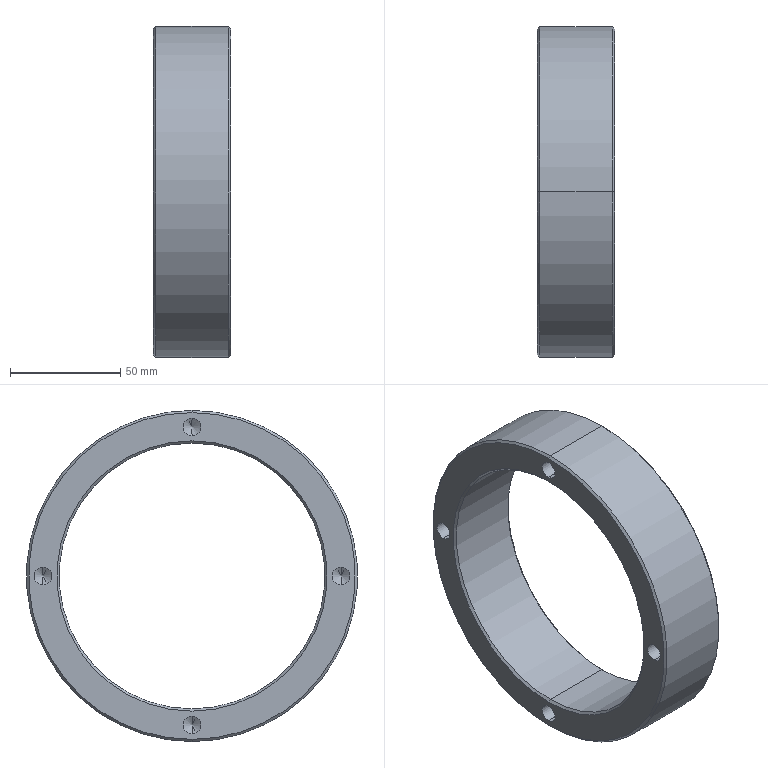Part | SolidWorks | features Chamfer 1, Extrusion 1, HoleWzd 1 | 1 solid | 30 faces | box 35 x 150 x 150 mm | volume 215991 mm3 | cone 16 | cylinder 12 | plane 2 | commonest cylinder face diameters 8 x8 120.4 x2 150 x2
STEP:
#1=CARTESIAN_POINT('',(15.,67.5,-4.));
#2=VERTEX_POINT('',#1);
#3=CARTESIAN_POINT('',(15.,67.5,4.));
#4=VERTEX_POINT('',#3);
#5=CARTESIAN_POINT('',(15.,67.5,0.));
#6=DIRECTION('',(-1.,0.,0.));
#7=DIRECTION('',(0.,0.,1.));
#8=AXIS2_PLACEMENT_3D('',#5,#6,#7);
#9=CIRCLE('',#8,4.);
#10=EDGE_CURVE('',#2,#4,#9,.T.);
#11=ORIENTED_EDGE('',*,*,#10,.F.);
#12=CARTESIAN_POINT('',(0.,67.5,-4.));
#13=VERTEX_POINT('',#12);
#14=CARTESIAN_POINT('',(0.,67.5,-4.));
#15=DIRECTION('',(-1.,0.,0.));
#16=VECTOR('',#15,1000.);
#17=LINE('',#14,#16);
#18=EDGE_CURVE('',#2,#13,#17,.T.);
#19=ORIENTED_EDGE('',*,*,#18,.T.);
#20=CARTESIAN_POINT('',(0.,67.5,4.));
#21=VERTEX_POINT('',#20);
#22=CARTESIAN_POINT('',(0.,67.5,0.));
#23=DIRECTION('',(-1.,0.,0.));
#24=DIRECTION('',(0.,0.,1.));
#25=AXIS2_PLACEMENT_3D('',#22,#23,#24);
#26=CIRCLE('',#25,4.);
#27=EDGE_CURVE('',#13,#21,#26,.T.);
#28=ORIENTED_EDGE('',*,*,#27,.T.);
#29=CARTESIAN_POINT('',(0.,67.5,4.));
#30=DIRECTION('',(-1.,0.,0.));
#31=VECTOR('',#30,1000.);
#32=LINE('',#29,#31);
#33=EDGE_CURVE('',#4,#21,#32,.T.);
#34=ORIENTED_EDGE('',*,*,#33,.F.);
#35=EDGE_LOOP('',(#11,#19,#28,#34));
#36=FACE_OUTER_BOUND('',#35,.T.);
#37=CARTESIAN_POINT('',(0.,67.5,0.));
#38=DIRECTION('',(-1.,0.,0.));
#39=DIRECTION('',(0.,0.,1.));
#40=AXIS2_PLACEMENT_3D('',#37,#38,#39);
#41=CYLINDRICAL_SURFACE('',#40,4.);
#42=ADVANCED_FACE('',(#36),#41,.F.);
#43=CARTESIAN_POINT('',(17.403,67.5,0.));
#44=VERTEX_POINT('',#43);
#45=CARTESIAN_POINT('',(15.,67.5,4.));
#46=DIRECTION('',(-0.515,0.,0.8572));
#47=VECTOR('',#46,1000.);
#48=LINE('',#45,#47);
#49=EDGE_CURVE('',#44,#4,#48,.T.);
#50=ORIENTED_EDGE('',*,*,#49,.F.);
#51=CARTESIAN_POINT('',(15.,67.5,-4.));
#52=DIRECTION('',(-0.515,0.,-0.8572));
#53=VECTOR('',#52,1000.);
#54=LINE('',#51,#53);
#55=EDGE_CURVE('',#44,#2,#54,.T.);
#56=ORIENTED_EDGE('',*,*,#55,.T.);
#57=ORIENTED_EDGE('',*,*,#10,.T.);
#58=EDGE_LOOP('',(#50,#56,#57));
#59=FACE_OUTER_BOUND('',#58,.T.);
#60=CARTESIAN_POINT('',(15.,67.5,0.));
#61=DIRECTION('',(-1.,0.,0.));
#62=DIRECTION('',(0.,0.,1.));
#63=AXIS2_PLACEMENT_3D('',#60,#61,#62);
#64=CONICAL_SURFACE('',#63,4.,1.03);
#65=ADVANCED_FACE('',(#59),#64,.F.);
#66=CARTESIAN_POINT('',(15.,0.,63.5));
#67=VERTEX_POINT('',#66);
#68=CARTESIAN_POINT('',(15.,0.,71.5));
#69=VERTEX_POINT('',#68);
#70=CARTESIAN_POINT('',(15.,0.,67.5));
#71=DIRECTION('',(-1.,0.,0.));
#72=DIRECTION('',(0.,0.,1.));
#73=AXIS2_PLACEMENT_3D('',#70,#71,#72);
#74=CIRCLE('',#73,4.);
#75=EDGE_CURVE('',#67,#69,#74,.T.);
#76=ORIENTED_EDGE('',*,*,#75,.F.);
#77=CARTESIAN_POINT('',(0.,0.,63.5));
#78=VERTEX_POINT('',#77);
#79=CARTESIAN_POINT('',(0.,0.,63.5));
#80=DIRECTION('',(-1.,0.,0.));
#81=VECTOR('',#80,1000.);
#82=LINE('',#79,#81);
#83=EDGE_CURVE('',#67,#78,#82,.T.);
#84=ORIENTED_EDGE('',*,*,#83,.T.);
#85=CARTESIAN_POINT('',(0.,0.,71.5));
#86=VERTEX_POINT('',#85);
#87=CARTESIAN_POINT('',(0.,0.,67.5));
#88=DIRECTION('',(-1.,0.,0.));
#89=DIRECTION('',(0.,0.,1.));
#90=AXIS2_PLACEMENT_3D('',#87,#88,#89);
#91=CIRCLE('',#90,4.);
#92=EDGE_CURVE('',#78,#86,#91,.T.);
#93=ORIENTED_EDGE('',*,*,#92,.T.);
#94=CARTESIAN_POINT('',(0.,0.,71.5));
#95=DIRECTION('',(-1.,0.,0.));
#96=VECTOR('',#95,1000.);
#97=LINE('',#94,#96);
#98=EDGE_CURVE('',#69,#86,#97,.T.);
#99=ORIENTED_EDGE('',*,*,#98,.F.);
#100=EDGE_LOOP('',(#76,#84,#93,#99));
#101=FACE_OUTER_BOUND('',#100,.T.);
#102=CARTESIAN_POINT('',(0.,0.,67.5));
#103=DIRECTION('',(-1.,0.,0.));
#104=DIRECTION('',(0.,0.,1.));
#105=AXIS2_PLACEMENT_3D('',#102,#103,#104);
#106=CYLINDRICAL_SURFACE('',#105,4.);
#107=ADVANCED_FACE('',(#101),#106,.F.);
#108=CARTESIAN_POINT('',(17.403,0.,67.5));
#109=VERTEX_POINT('',#108);
#110=CARTESIAN_POINT('',(15.,0.,71.5));
#111=DIRECTION('',(-0.515,0.,0.8572));
#112=VECTOR('',#111,1000.);
#113=LINE('',#110,#112);
#114=EDGE_CURVE('',#109,#69,#113,.T.);
#115=ORIENTED_EDGE('',*,*,#114,.F.);
#116=CARTESIAN_POINT('',(15.,0.,63.5));
#117=DIRECTION('',(-0.515,0.,-0.8572));
#118=VECTOR('',#117,1000.);
#119=LINE('',#116,#118);
#120=EDGE_CURVE('',#109,#67,#119,.T.);
#121=ORIENTED_EDGE('',*,*,#120,.T.);
#122=ORIENTED_EDGE('',*,*,#75,.T.);
#123=EDGE_LOOP('',(#115,#121,#122));
#124=FACE_OUTER_BOUND('',#123,.T.);
#125=CARTESIAN_POINT('',(15.,0.,67.5));
#126=DIRECTION('',(-1.,0.,0.));
#127=DIRECTION('',(0.,0.,1.));
#128=AXIS2_PLACEMENT_3D('',#125,#126,#127);
#129=CONICAL_SURFACE('',#128,4.,1.03);
#130=ADVANCED_FACE('',(#124),#129,.F.);
#131=CARTESIAN_POINT('',(15.,-67.5,-4.));
#132=VERTEX_POINT('',#131);
#133=CARTESIAN_POINT('',(15.,-67.5,4.));
#134=VERTEX_POINT('',#133);
#135=CARTESIAN_POINT('',(15.,-67.5,0.));
#136=DIRECTION('',(-1.,0.,0.));
#137=DIRECTION('',(0.,0.,1.));
#138=AXIS2_PLACEMENT_3D('',#135,#136,#137);
#139=CIRCLE('',#138,4.);
#140=EDGE_CURVE('',#132,#134,#139,.T.);
#141=ORIENTED_EDGE('',*,*,#140,.F.);
#142=CARTESIAN_POINT('',(0.,-67.5,-4.));
#143=VERTEX_POINT('',#142);
#144=CARTESIAN_POINT('',(0.,-67.5,-4.));
#145=DIRECTION('',(-1.,0.,0.));
#146=VECTOR('',#145,1000.);
#147=LINE('',#144,#146);
#148=EDGE_CURVE('',#132,#143,#147,.T.);
#149=ORIENTED_EDGE('',*,*,#148,.T.);
#150=CARTESIAN_POINT('',(0.,-67.5,4.));
#151=VERTEX_POINT('',#150);
#152=CARTESIAN_POINT('',(0.,-67.5,0.));
#153=DIRECTION('',(-1.,0.,0.));
#154=DIRECTION('',(0.,0.,1.));
#155=AXIS2_PLACEMENT_3D('',#152,#153,#154);
#156=CIRCLE('',#155,4.);
#157=EDGE_CURVE('',#143,#151,#156,.T.);
#158=ORIENTED_EDGE('',*,*,#157,.T.);
#159=CARTESIAN_POINT('',(0.,-67.5,4.));
#160=DIRECTION('',(-1.,0.,0.));
#161=VECTOR('',#160,1000.);
#162=LINE('',#159,#161);
#163=EDGE_CURVE('',#134,#151,#162,.T.);
#164=ORIENTED_EDGE('',*,*,#163,.F.);
#165=EDGE_LOOP('',(#141,#149,#158,#164));
#166=FACE_OUTER_BOUND('',#165,.T.);
#167=CARTESIAN_POINT('',(0.,-67.5,0.));
#168=DIRECTION('',(-1.,0.,0.));
#169=DIRECTION('',(0.,0.,1.));
#170=AXIS2_PLACEMENT_3D('',#167,#168,#169);
#171=CYLINDRICAL_SURFACE('',#170,4.);
#172=ADVANCED_FACE('',(#166),#171,.F.);
#173=CARTESIAN_POINT('',(17.403,-67.5,0.));
#174=VERTEX_POINT('',#173);
#175=CARTESIAN_POINT('',(15.,-67.5,4.));
#176=DIRECTION('',(-0.515,0.,0.8572));
#177=VECTOR('',#176,1000.);
#178=LINE('',#175,#177);
#179=EDGE_CURVE('',#174,#134,#178,.T.);
#180=ORIENTED_EDGE('',*,*,#179,.F.);
#181=CARTESIAN_POINT('',(15.,-67.5,-4.));
#182=DIRECTION('',(-0.515,0.,-0.8572));
#183=VECTOR('',#182,1000.);
#184=LINE('',#181,#183);
#185=EDGE_CURVE('',#174,#132,#184,.T.);
#186=ORIENTED_EDGE('',*,*,#185,.T.);
#187=ORIENTED_EDGE('',*,*,#140,.T.);
#188=EDGE_LOOP('',(#180,#186,#187));
#189=FACE_OUTER_BOUND('',#188,.T.);
#190=CARTESIAN_POINT('',(15.,-67.5,0.));
#191=DIRECTION('',(-1.,0.,0.));
#192=DIRECTION('',(0.,0.,1.));
#193=AXIS2_PLACEMENT_3D('',#190,#191,#192);
#194=CONICAL_SURFACE('',#193,4.,1.03);
#195=ADVANCED_FACE('',(#189),#194,.F.);
#196=CARTESIAN_POINT('',(15.,0.,-71.5));
#197=VERTEX_POINT('',#196);
#198=CARTESIAN_POINT('',(15.,0.,-63.5));
#199=VERTEX_POINT('',#198);
#200=CARTESIAN_POINT('',(15.,0.,-67.5));
#201=DIRECTION('',(-1.,0.,0.));
#202=DIRECTION('',(0.,0.,1.));
#203=AXIS2_PLACEMENT_3D('',#200,#201,#202);
#204=CIRCLE('',#203,4.);
#205=EDGE_CURVE('',#197,#199,#204,.T.);
#206=ORIENTED_EDGE('',*,*,#205,.F.);
#207=CARTESIAN_POINT('',(0.,0.,-71.5));
#208=VERTEX_POINT('',#207);
#209=CARTESIAN_POINT('',(0.,0.,-71.5));
#210=DIRECTION('',(-1.,0.,0.));
#211=VECTOR('',#210,1000.);
#212=LINE('',#209,#211);
#213=EDGE_CURVE('',#197,#208,#212,.T.);
#214=ORIENTED_EDGE('',*,*,#213,.T.);
#215=CARTESIAN_POINT('',(0.,0.,-63.5));
#216=VERTEX_POINT('',#215);
#217=CARTESIAN_POINT('',(0.,0.,-67.5));
#218=DIRECTION('',(-1.,0.,0.));
#219=DIRECTION('',(0.,0.,1.));
#220=AXIS2_PLACEMENT_3D('',#217,#218,#219);
#221=CIRCLE('',#220,4.);
#222=EDGE_CURVE('',#208,#216,#221,.T.);
#223=ORIENTED_EDGE('',*,*,#222,.T.);
#224=CARTESIAN_POINT('',(0.,0.,-63.5));
#225=DIRECTION('',(-1.,0.,0.));
#226=VECTOR('',#225,1000.);
#227=LINE('',#224,#226);
#228=EDGE_CURVE('',#199,#216,#227,.T.);
#229=ORIENTED_EDGE('',*,*,#228,.F.);
#230=EDGE_LOOP('',(#206,#214,#223,#229));
#231=FACE_OUTER_BOUND('',#230,.T.);
#232=CARTESIAN_POINT('',(0.,0.,-67.5));
#233=DIRECTION('',(-1.,0.,0.));
#234=DIRECTION('',(0.,0.,1.));
#235=AXIS2_PLACEMENT_3D('',#232,#233,#234);
#236=CYLINDRICAL_SURFACE('',#235,4.);
#237=ADVANCED_FACE('',(#231),#236,.F.);
#238=CARTESIAN_POINT('',(17.403,0.,-67.5));
#239=VERTEX_POINT('',#238);
#240=CARTESIAN_POINT('',(15.,0.,-63.5));
#241=DIRECTION('',(-0.515,0.,0.8572));
#242=VECTOR('',#241,1000.);
#243=LINE('',#240,#242);
#244=EDGE_CURVE('',#239,#199,#243,.T.);
#245=ORIENTED_EDGE('',*,*,#244,.F.);
#246=CARTESIAN_POINT('',(15.,0.,-71.5));
#247=DIRECTION('',(-0.515,0.,-0.8572));
#248=VECTOR('',#247,1000.);
#249=LINE('',#246,#248);
#250=EDGE_CURVE('',#239,#197,#249,.T.);
#251=ORIENTED_EDGE('',*,*,#250,.T.);
#252=ORIENTED_EDGE('',*,*,#205,.T.);
#253=EDGE_LOOP('',(#245,#251,#252));
#254=FACE_OUTER_BOUND('',#253,.T.);
#255=CARTESIAN_POINT('',(15.,0.,-67.5));
#256=DIRECTION('',(-1.,0.,0.));
#257=DIRECTION('',(0.,0.,1.));
#258=AXIS2_PLACEMENT_3D('',#255,#256,#257);
#259=CONICAL_SURFACE('',#258,4.,1.03);
#260=ADVANCED_FACE('',(#254),#259,.F.);
#261=CARTESIAN_POINT('',(35.,0.,-74.));
#262=VERTEX_POINT('',#261);
#263=CARTESIAN_POINT('',(35.,0.,74.));
#264=VERTEX_POINT('',#263);
#265=CARTESIAN_POINT('',(35.,0.,0.));
#266=DIRECTION('',(1.,0.,0.));
#267=DIRECTION('',(0.,0.,-1.));
#268=AXIS2_PLACEMENT_3D('',#265,#266,#267);
#269=CIRCLE('',#268,74.);
#270=EDGE_CURVE('',#262,#264,#269,.T.);
#271=ORIENTED_EDGE('',*,*,#270,.F.);
#272=CARTESIAN_POINT('',(34.,0.,-75.));
#273=VERTEX_POINT('',#272);
#274=CARTESIAN_POINT('',(35.,0.,-74.));
#275=DIRECTION('',(-0.7071,0.,-0.7071));
#276=VECTOR('',#275,1000.);
#277=LINE('',#274,#276);
#278=EDGE_CURVE('',#262,#273,#277,.T.);
#279=ORIENTED_EDGE('',*,*,#278,.T.);
#280=CARTESIAN_POINT('',(34.,0.,75.));
#281=VERTEX_POINT('',#280);
#282=CARTESIAN_POINT('',(34.,0.,0.));
#283=DIRECTION('',(-1.,0.,0.));
#284=DIRECTION('',(0.,0.,-1.));
#285=AXIS2_PLACEMENT_3D('',#282,#283,#284);
#286=CIRCLE('',#285,75.);
#287=EDGE_CURVE('',#281,#273,#286,.T.);
#288=ORIENTED_EDGE('',*,*,#287,.F.);
#289=CARTESIAN_POINT('',(35.,0.,74.));
#290=DIRECTION('',(-0.7071,0.,0.7071));
#291=VECTOR('',#290,1000.);
#292=LINE('',#289,#291);
#293=EDGE_CURVE('',#264,#281,#292,.T.);
#294=ORIENTED_EDGE('',*,*,#293,.F.);
#295=EDGE_LOOP('',(#271,#279,#288,#294));
#296=FACE_OUTER_BOUND('',#295,.T.);
#297=CARTESIAN_POINT('',(35.,0.,0.));
#298=DIRECTION('',(-1.,0.,0.));
#299=DIRECTION('',(0.,0.,1.));
#300=AXIS2_PLACEMENT_3D('',#297,#298,#299);
#301=CONICAL_SURFACE('',#300,74.,0.7854);
#302=ADVANCED_FACE('',(#296),#301,.T.);
#303=CARTESIAN_POINT('',(34.,0.,60.2));
#304=VERTEX_POINT('',#303);
#305=CARTESIAN_POINT('',(34.,0.,-60.2));
#306=VERTEX_POINT('',#305);
#307=CARTESIAN_POINT('',(34.,0.,0.));
#308=DIRECTION('',(1.,0.,0.));
#309=DIRECTION('',(0.,0.,-1.));
#310=AXIS2_PLACEMENT_3D('',#307,#308,#309);
#311=CIRCLE('',#310,60.2);
#312=EDGE_CURVE('',#304,#306,#311,.T.);
#313=ORIENTED_EDGE('',*,*,#312,.F.);
#314=CARTESIAN_POINT('',(35.,0.,61.2));
#315=VERTEX_POINT('',#314);
#316=CARTESIAN_POINT('',(34.,0.,60.2));
#317=DIRECTION('',(0.7071,0.,0.7071));
#318=VECTOR('',#317,1000.);
#319=LINE('',#316,#318);
#320=EDGE_CURVE('',#304,#315,#319,.T.);
#321=ORIENTED_EDGE('',*,*,#320,.T.);
#322=CARTESIAN_POINT('',(35.,0.,-61.2));
#323=VERTEX_POINT('',#322);
#324=CARTESIAN_POINT('',(35.,0.,0.));
#325=DIRECTION('',(-1.,0.,0.));
#326=DIRECTION('',(0.,0.,-1.));
#327=AXIS2_PLACEMENT_3D('',#324,#325,#326);
#328=CIRCLE('',#327,61.2);
#329=EDGE_CURVE('',#323,#315,#328,.T.);
#330=ORIENTED_EDGE('',*,*,#329,.F.);
#331=CARTESIAN_POINT('',(34.,0.,-60.2));
#332=DIRECTION('',(0.7071,0.,-0.7071));
#333=VECTOR('',#332,1000.);
#334=LINE('',#331,#333);
#335=EDGE_CURVE('',#306,#323,#334,.T.);
#336=ORIENTED_EDGE('',*,*,#335,.F.);
#337=EDGE_LOOP('',(#313,#321,#330,#336));
#338=FACE_OUTER_BOUND('',#337,.T.);
#339=CARTESIAN_POINT('',(34.,0.,0.));
#340=DIRECTION('',(1.,0.,0.));
#341=DIRECTION('',(0.,0.,-1.));
#342=AXIS2_PLACEMENT_3D('',#339,#340,#341);
#343=CONICAL_SURFACE('',#342,60.2,0.7854);
#344=ADVANCED_FACE('',(#338),#343,.F.);
#345=CARTESIAN_POINT('',(0.,0.,74.));
#346=VERTEX_POINT('',#345);
#347=CARTESIAN_POINT('',(0.,0.,-74.));
#348=VERTEX_POINT('',#347);
#349=CARTESIAN_POINT('',(0.,0.,0.));
#350=DIRECTION('',(-1.,0.,0.));
#351=DIRECTION('',(0.,0.,-1.));
#352=AXIS2_PLACEMENT_3D('',#349,#350,#351);
#353=CIRCLE('',#352,74.);
#354=EDGE_CURVE('',#346,#348,#353,.T.);
#355=ORIENTED_EDGE('',*,*,#354,.F.);
#356=CARTESIAN_POINT('',(1.,0.,75.));
#357=VERTEX_POINT('',#356);
#358=CARTESIAN_POINT('',(1.,0.,75.));
#359=DIRECTION('',(0.7071,0.,0.7071));
#360=VECTOR('',#359,1000.);
#361=LINE('',#358,#360);
#362=EDGE_CURVE('',#346,#357,#361,.T.);
#363=ORIENTED_EDGE('',*,*,#362,.T.);
#364=CARTESIAN_POINT('',(1.,0.,-75.));
#365=VERTEX_POINT('',#364);
#366=CARTESIAN_POINT('',(1.,0.,0.));
#367=DIRECTION('',(1.,0.,0.));
#368=DIRECTION('',(0.,0.,-1.));
#369=AXIS2_PLACEMENT_3D('',#366,#367,#368);
#370=CIRCLE('',#369,75.);
#371=EDGE_CURVE('',#365,#357,#370,.T.);
#372=ORIENTED_EDGE('',*,*,#371,.F.);
#373=CARTESIAN_POINT('',(1.,0.,-75.));
#374=DIRECTION('',(0.7071,0.,-0.7071));
#375=VECTOR('',#374,1000.);
#376=LINE('',#373,#375);
#377=EDGE_CURVE('',#348,#365,#376,.T.);
#378=ORIENTED_EDGE('',*,*,#377,.F.);
#379=EDGE_LOOP('',(#355,#363,#372,#378));
#380=FACE_OUTER_BOUND('',#379,.T.);
#381=CARTESIAN_POINT('',(1.,0.,0.));
#382=DIRECTION('',(1.,0.,0.));
#383=DIRECTION('',(0.,0.,-1.));
#384=AXIS2_PLACEMENT_3D('',#381,#382,#383);
#385=CONICAL_SURFACE('',#384,75.,0.7854);
#386=ADVANCED_FACE('',(#380),#385,.T.);
#387=CARTESIAN_POINT('',(1.,0.,-60.2));
#388=VERTEX_POINT('',#387);
#389=CARTESIAN_POINT('',(1.,0.,60.2));
#390=VERTEX_POINT('',#389);
#391=CARTESIAN_POINT('',(1.,0.,0.));
#392=DIRECTION('',(-1.,0.,0.));
#393=DIRECTION('',(0.,0.,-1.));
#394=AXIS2_PLACEMENT_3D('',#391,#392,#393);
#395=CIRCLE('',#394,60.2);
#396=EDGE_CURVE('',#388,#390,#395,.T.);
#397=ORIENTED_EDGE('',*,*,#396,.F.);
#398=CARTESIAN_POINT('',(0.,0.,-61.2));
#399=VERTEX_POINT('',#398);
#400=CARTESIAN_POINT('',(0.,0.,-61.2));
#401=DIRECTION('',(-0.7071,0.,-0.7071));
#402=VECTOR('',#401,1000.);
#403=LINE('',#400,#402);
#404=EDGE_CURVE('',#388,#399,#403,.T.);
#405=ORIENTED_EDGE('',*,*,#404,.T.);
#406=CARTESIAN_POINT('',(0.,0.,61.2));
#407=VERTEX_POINT('',#406);
#408=CARTESIAN_POINT('',(0.,0.,0.));
#409=DIRECTION('',(1.,0.,0.));
#410=DIRECTION('',(0.,0.,-1.));
#411=AXIS2_PLACEMENT_3D('',#408,#409,#410);
#412=CIRCLE('',#411,61.2);
#413=EDGE_CURVE('',#407,#399,#412,.T.);
#414=ORIENTED_EDGE('',*,*,#413,.F.);
#415=CARTESIAN_POINT('',(0.,0.,61.2));
#416=DIRECTION('',(-0.7071,0.,0.7071));
#417=VECTOR('',#416,1000.);
#418=LINE('',#415,#417);
#419=EDGE_CURVE('',#390,#407,#418,.T.);
#420=ORIENTED_EDGE('',*,*,#419,.F.);
#421=EDGE_LOOP('',(#397,#405,#414,#420));
#422=FACE_OUTER_BOUND('',#421,.T.);
#423=CARTESIAN_POINT('',(0.,0.,0.));
#424=DIRECTION('',(-1.,0.,0.));
#425=DIRECTION('',(0.,0.,1.));
#426=AXIS2_PLACEMENT_3D('',#423,#424,#425);
#427=CONICAL_SURFACE('',#426,61.2,0.7854);
#428=ADVANCED_FACE('',(#422),#427,.F.);
#429=ORIENTED_EDGE('',*,*,#312,.T.);
#430=CARTESIAN_POINT('',(35.,0.,-60.2));
#431=DIRECTION('',(-1.,0.,0.));
#432=VECTOR('',#431,1000.);
#433=LINE('',#430,#432);
#434=EDGE_CURVE('',#306,#388,#433,.T.);
#435=ORIENTED_EDGE('',*,*,#434,.T.);
#436=ORIENTED_EDGE('',*,*,#396,.T.);
#437=CARTESIAN_POINT('',(35.,0.,60.2));
#438=DIRECTION('',(-1.,0.,0.));
#439=VECTOR('',#438,1000.);
#440=LINE('',#437,#439);
#441=EDGE_CURVE('',#304,#390,#440,.T.);
#442=ORIENTED_EDGE('',*,*,#441,.F.);
#443=EDGE_LOOP('',(#429,#435,#436,#442));
#444=FACE_OUTER_BOUND('',#443,.T.);
#445=CARTESIAN_POINT('',(35.,0.,0.));
#446=DIRECTION('',(-1.,0.,0.));
#447=DIRECTION('',(0.,0.,1.));
#448=AXIS2_PLACEMENT_3D('',#445,#446,#447);
#449=CYLINDRICAL_SURFACE('',#448,60.2);
#450=ADVANCED_FACE('',(#444),#449,.F.);
#451=ORIENTED_EDGE('',*,*,#287,.T.);
#452=CARTESIAN_POINT('',(35.,0.,-75.));
#453=DIRECTION('',(-1.,0.,0.));
#454=VECTOR('',#453,1000.);
#455=LINE('',#452,#454);
#456=EDGE_CURVE('',#273,#365,#455,.T.);
#457=ORIENTED_EDGE('',*,*,#456,.T.);
#458=ORIENTED_EDGE('',*,*,#371,.T.);
#459=CARTESIAN_POINT('',(35.,0.,75.));
#460=DIRECTION('',(-1.,0.,0.));
#461=VECTOR('',#460,1000.);
#462=LINE('',#459,#461);
#463=EDGE_CURVE('',#281,#357,#462,.T.);
#464=ORIENTED_EDGE('',*,*,#463,.F.);
#465=EDGE_LOOP('',(#451,#457,#458,#464));
#466=FACE_OUTER_BOUND('',#465,.T.);
#467=CARTESIAN_POINT('',(35.,0.,0.));
#468=DIRECTION('',(-1.,0.,0.));
#469=DIRECTION('',(0.,0.,1.));
#470=AXIS2_PLACEMENT_3D('',#467,#468,#469);
#471=CYLINDRICAL_SURFACE('',#470,75.);
#472=ADVANCED_FACE('',(#466),#471,.T.);
#473=ORIENTED_EDGE('',*,*,#329,.T.);
#474=CARTESIAN_POINT('',(35.,0.,0.));
#475=DIRECTION('',(-1.,0.,0.));
#476=DIRECTION('',(0.,0.,-1.));
#477=AXIS2_PLACEMENT_3D('',#474,#475,#476);
#478=CIRCLE('',#477,61.2);
#479=EDGE_CURVE('',#315,#323,#478,.T.);
#480=ORIENTED_EDGE('',*,*,#479,.T.);
#481=EDGE_LOOP('',(#473,#480));
#482=FACE_BOUND('',#481,.T.);
#483=CARTESIAN_POINT('',(35.,0.,0.));
#484=DIRECTION('',(1.,0.,0.));
#485=DIRECTION('',(0.,0.,-1.));
#486=AXIS2_PLACEMENT_3D('',#483,#484,#485);
#487=CIRCLE('',#486,74.);
#488=EDGE_CURVE('',#264,#262,#487,.T.);
#489=ORIENTED_EDGE('',*,*,#488,.T.);
#490=ORIENTED_EDGE('',*,*,#270,.T.);
#491=EDGE_LOOP('',(#489,#490));
#492=FACE_OUTER_BOUND('',#491,.T.);
#493=CARTESIAN_POINT('',(35.,0.,0.));
#494=DIRECTION('',(1.,0.,0.));
#495=DIRECTION('',(0.,0.,-1.));
#496=AXIS2_PLACEMENT_3D('',#493,#494,#495);
#497=PLANE('',#496);
#498=ADVANCED_FACE('',(#482,#492),#497,.T.);
#499=CARTESIAN_POINT('',(0.,67.5,0.));
#500=DIRECTION('',(-1.,0.,0.));
#501=DIRECTION('',(0.,0.,1.));
#502=AXIS2_PLACEMENT_3D('',#499,#500,#501);
#503=CIRCLE('',#502,4.);
#504=EDGE_CURVE('',#21,#13,#503,.T.);
#505=ORIENTED_EDGE('',*,*,#504,.F.);
#506=ORIENTED_EDGE('',*,*,#27,.F.);
#507=EDGE_LOOP('',(#505,#506));
#508=FACE_BOUND('',#507,.T.);
#509=CARTESIAN_POINT('',(0.,0.,67.5));
#510=DIRECTION('',(-1.,0.,0.));
#511=DIRECTION('',(0.,0.,1.));
#512=AXIS2_PLACEMENT_3D('',#509,#510,#511);
#513=CIRCLE('',#512,4.);
#514=EDGE_CURVE('',#86,#78,#513,.T.);
#515=ORIENTED_EDGE('',*,*,#514,.F.);
#516=ORIENTED_EDGE('',*,*,#92,.F.);
#517=EDGE_LOOP('',(#515,#516));
#518=FACE_BOUND('',#517,.T.);
#519=CARTESIAN_POINT('',(0.,-67.5,0.));
#520=DIRECTION('',(-1.,0.,0.));
#521=DIRECTION('',(0.,0.,1.));
#522=AXIS2_PLACEMENT_3D('',#519,#520,#521);
#523=CIRCLE('',#522,4.);
#524=EDGE_CURVE('',#151,#143,#523,.T.);
#525=ORIENTED_EDGE('',*,*,#524,.F.);
#526=ORIENTED_EDGE('',*,*,#157,.F.);
#527=EDGE_LOOP('',(#525,#526));
#528=FACE_BOUND('',#527,.T.);
#529=CARTESIAN_POINT('',(0.,0.,-67.5));
#530=DIRECTION('',(-1.,0.,0.));
#531=DIRECTION('',(0.,0.,1.));
#532=AXIS2_PLACEMENT_3D('',#529,#530,#531);
#533=CIRCLE('',#532,4.);
#534=EDGE_CURVE('',#216,#208,#533,.T.);
#535=ORIENTED_EDGE('',*,*,#534,.F.);
#536=ORIENTED_EDGE('',*,*,#222,.F.);
#537=EDGE_LOOP('',(#535,#536));
#538=FACE_BOUND('',#537,.T.);
#539=ORIENTED_EDGE('',*,*,#413,.T.);
#540=CARTESIAN_POINT('',(0.,0.,0.));
#541=DIRECTION('',(1.,0.,0.));
#542=DIRECTION('',(0.,0.,-1.));
#543=AXIS2_PLACEMENT_3D('',#540,#541,#542);
#544=CIRCLE('',#543,61.2);
#545=EDGE_CURVE('',#399,#407,#544,.T.);
#546=ORIENTED_EDGE('',*,*,#545,.T.);
#547=EDGE_LOOP('',(#539,#546));
#548=FACE_BOUND('',#547,.T.);
#549=CARTESIAN_POINT('',(0.,0.,0.));
#550=DIRECTION('',(-1.,0.,0.));
#551=DIRECTION('',(0.,0.,-1.));
#552=AXIS2_PLACEMENT_3D('',#549,#550,#551);
#553=CIRCLE('',#552,74.);
#554=EDGE_CURVE('',#348,#346,#553,.T.);
#555=ORIENTED_EDGE('',*,*,#554,.T.);
#556=ORIENTED_EDGE('',*,*,#354,.T.);
#557=EDGE_LOOP('',(#555,#556));
#558=FACE_OUTER_BOUND('',#557,.T.);
#559=CARTESIAN_POINT('',(0.,0.,0.));
#560=DIRECTION('',(1.,0.,0.));
#561=DIRECTION('',(0.,0.,-1.));
#562=AXIS2_PLACEMENT_3D('',#559,#560,#561);
#563=PLANE('',#562);
#564=ADVANCED_FACE('',(#508,#518,#528,#538,#548,#558),#563,.F.);
#565=ORIENTED_EDGE('',*,*,#456,.F.);
#566=CARTESIAN_POINT('',(34.,0.,0.));
#567=DIRECTION('',(-1.,0.,0.));
#568=DIRECTION('',(0.,0.,-1.));
#569=AXIS2_PLACEMENT_3D('',#566,#567,#568);
#570=CIRCLE('',#569,75.);
#571=EDGE_CURVE('',#273,#281,#570,.T.);
#572=ORIENTED_EDGE('',*,*,#571,.T.);
#573=ORIENTED_EDGE('',*,*,#463,.T.);
#574=CARTESIAN_POINT('',(1.,0.,0.));
#575=DIRECTION('',(1.,0.,0.));
#576=DIRECTION('',(0.,0.,-1.));
#577=AXIS2_PLACEMENT_3D('',#574,#575,#576);
#578=CIRCLE('',#577,75.);
#579=EDGE_CURVE('',#357,#365,#578,.T.);
#580=ORIENTED_EDGE('',*,*,#579,.T.);
#581=EDGE_LOOP('',(#565,#572,#573,#580));
#582=FACE_OUTER_BOUND('',#581,.T.);
#583=CARTESIAN_POINT('',(35.,0.,0.));
#584=DIRECTION('',(-1.,0.,0.));
#585=DIRECTION('',(0.,0.,1.));
#586=AXIS2_PLACEMENT_3D('',#583,#584,#585);
#587=CYLINDRICAL_SURFACE('',#586,75.);
#588=ADVANCED_FACE('',(#582),#587,.T.);
#589=ORIENTED_EDGE('',*,*,#434,.F.);
#590=CARTESIAN_POINT('',(34.,0.,0.));
#591=DIRECTION('',(1.,0.,0.));
#592=DIRECTION('',(0.,0.,-1.));
#593=AXIS2_PLACEMENT_3D('',#590,#591,#592);
#594=CIRCLE('',#593,60.2);
#595=EDGE_CURVE('',#306,#304,#594,.T.);
#596=ORIENTED_EDGE('',*,*,#595,.T.);
#597=ORIENTED_EDGE('',*,*,#441,.T.);
#598=CARTESIAN_POINT('',(1.,0.,0.));
#599=DIRECTION('',(-1.,0.,0.));
#600=DIRECTION('',(0.,0.,-1.));
#601=AXIS2_PLACEMENT_3D('',#598,#599,#600);
#602=CIRCLE('',#601,60.2);
#603=EDGE_CURVE('',#390,#388,#602,.T.);
#604=ORIENTED_EDGE('',*,*,#603,.T.);
#605=EDGE_LOOP('',(#589,#596,#597,#604));
#606=FACE_OUTER_BOUND('',#605,.T.);
#607=CARTESIAN_POINT('',(35.,0.,0.));
#608=DIRECTION('',(-1.,0.,0.));
#609=DIRECTION('',(0.,0.,1.));
#610=AXIS2_PLACEMENT_3D('',#607,#608,#609);
#611=CYLINDRICAL_SURFACE('',#610,60.2);
#612=ADVANCED_FACE('',(#606),#611,.F.);
#613=ORIENTED_EDGE('',*,*,#404,.F.);
#614=ORIENTED_EDGE('',*,*,#603,.F.);
#615=ORIENTED_EDGE('',*,*,#419,.T.);
#616=ORIENTED_EDGE('',*,*,#545,.F.);
#617=EDGE_LOOP('',(#613,#614,#615,#616));
#618=FACE_OUTER_BOUND('',#617,.T.);
#619=CARTESIAN_POINT('',(0.,0.,0.));
#620=DIRECTION('',(-1.,0.,0.));
#621=DIRECTION('',(0.,0.,1.));
#622=AXIS2_PLACEMENT_3D('',#619,#620,#621);
#623=CONICAL_SURFACE('',#622,61.2,0.7854);
#624=ADVANCED_FACE('',(#618),#623,.F.);
#625=ORIENTED_EDGE('',*,*,#362,.F.);
#626=ORIENTED_EDGE('',*,*,#554,.F.);
#627=ORIENTED_EDGE('',*,*,#377,.T.);
#628=ORIENTED_EDGE('',*,*,#579,.F.);
#629=EDGE_LOOP('',(#625,#626,#627,#628));
#630=FACE_OUTER_BOUND('',#629,.T.);
#631=CARTESIAN_POINT('',(1.,0.,0.));
#632=DIRECTION('',(1.,0.,0.));
#633=DIRECTION('',(0.,0.,-1.));
#634=AXIS2_PLACEMENT_3D('',#631,#632,#633);
#635=CONICAL_SURFACE('',#634,75.,0.7854);
#636=ADVANCED_FACE('',(#630),#635,.T.);
#637=ORIENTED_EDGE('',*,*,#320,.F.);
#638=ORIENTED_EDGE('',*,*,#595,.F.);
#639=ORIENTED_EDGE('',*,*,#335,.T.);
#640=ORIENTED_EDGE('',*,*,#479,.F.);
#641=EDGE_LOOP('',(#637,#638,#639,#640));
#642=FACE_OUTER_BOUND('',#641,.T.);
#643=CARTESIAN_POINT('',(34.,0.,0.));
#644=DIRECTION('',(1.,0.,0.));
#645=DIRECTION('',(0.,0.,-1.));
#646=AXIS2_PLACEMENT_3D('',#643,#644,#645);
#647=CONICAL_SURFACE('',#646,60.2,0.7854);
#648=ADVANCED_FACE('',(#642),#647,.F.);
#649=ORIENTED_EDGE('',*,*,#278,.F.);
#650=ORIENTED_EDGE('',*,*,#488,.F.);
#651=ORIENTED_EDGE('',*,*,#293,.T.);
#652=ORIENTED_EDGE('',*,*,#571,.F.);
#653=EDGE_LOOP('',(#649,#650,#651,#652));
#654=FACE_OUTER_BOUND('',#653,.T.);
#655=CARTESIAN_POINT('',(35.,0.,0.));
#656=DIRECTION('',(-1.,0.,0.));
#657=DIRECTION('',(0.,0.,1.));
#658=AXIS2_PLACEMENT_3D('',#655,#656,#657);
#659=CONICAL_SURFACE('',#658,74.,0.7854);
#660=ADVANCED_FACE('',(#654),#659,.T.);
#661=ORIENTED_EDGE('',*,*,#250,.F.);
#662=ORIENTED_EDGE('',*,*,#244,.T.);
#663=CARTESIAN_POINT('',(15.,0.,-67.5));
#664=DIRECTION('',(-1.,0.,0.));
#665=DIRECTION('',(0.,0.,1.));
#666=AXIS2_PLACEMENT_3D('',#663,#664,#665);
#667=CIRCLE('',#666,4.);
#668=EDGE_CURVE('',#199,#197,#667,.T.);
#669=ORIENTED_EDGE('',*,*,#668,.T.);
#670=EDGE_LOOP('',(#661,#662,#669));
#671=FACE_OUTER_BOUND('',#670,.T.);
#672=CARTESIAN_POINT('',(15.,0.,-67.5));
#673=DIRECTION('',(-1.,0.,0.));
#674=DIRECTION('',(0.,0.,1.));
#675=AXIS2_PLACEMENT_3D('',#672,#673,#674);
#676=CONICAL_SURFACE('',#675,4.,1.03);
#677=ADVANCED_FACE('',(#671),#676,.F.);
#678=ORIENTED_EDGE('',*,*,#213,.F.);
#679=ORIENTED_EDGE('',*,*,#668,.F.);
#680=ORIENTED_EDGE('',*,*,#228,.T.);
#681=ORIENTED_EDGE('',*,*,#534,.T.);
#682=EDGE_LOOP('',(#678,#679,#680,#681));
#683=FACE_OUTER_BOUND('',#682,.T.);
#684=CARTESIAN_POINT('',(0.,0.,-67.5));
#685=DIRECTION('',(-1.,0.,0.));
#686=DIRECTION('',(0.,0.,1.));
#687=AXIS2_PLACEMENT_3D('',#684,#685,#686);
#688=CYLINDRICAL_SURFACE('',#687,4.);
#689=ADVANCED_FACE('',(#683),#688,.F.);
#690=ORIENTED_EDGE('',*,*,#185,.F.);
#691=ORIENTED_EDGE('',*,*,#179,.T.);
#692=CARTESIAN_POINT('',(15.,-67.5,0.));
#693=DIRECTION('',(-1.,0.,0.));
#694=DIRECTION('',(0.,0.,1.));
#695=AXIS2_PLACEMENT_3D('',#692,#693,#694);
#696=CIRCLE('',#695,4.);
#697=EDGE_CURVE('',#134,#132,#696,.T.);
#698=ORIENTED_EDGE('',*,*,#697,.T.);
#699=EDGE_LOOP('',(#690,#691,#698));
#700=FACE_OUTER_BOUND('',#699,.T.);
#701=CARTESIAN_POINT('',(15.,-67.5,0.));
#702=DIRECTION('',(-1.,0.,0.));
#703=DIRECTION('',(0.,0.,1.));
#704=AXIS2_PLACEMENT_3D('',#701,#702,#703);
#705=CONICAL_SURFACE('',#704,4.,1.03);
#706=ADVANCED_FACE('',(#700),#705,.F.);
#707=ORIENTED_EDGE('',*,*,#148,.F.);
#708=ORIENTED_EDGE('',*,*,#697,.F.);
#709=ORIENTED_EDGE('',*,*,#163,.T.);
#710=ORIENTED_EDGE('',*,*,#524,.T.);
#711=EDGE_LOOP('',(#707,#708,#709,#710));
#712=FACE_OUTER_BOUND('',#711,.T.);
#713=CARTESIAN_POINT('',(0.,-67.5,0.));
#714=DIRECTION('',(-1.,0.,0.));
#715=DIRECTION('',(0.,0.,1.));
#716=AXIS2_PLACEMENT_3D('',#713,#714,#715);
#717=CYLINDRICAL_SURFACE('',#716,4.);
#718=ADVANCED_FACE('',(#712),#717,.F.);
#719=ORIENTED_EDGE('',*,*,#120,.F.);
#720=ORIENTED_EDGE('',*,*,#114,.T.);
#721=CARTESIAN_POINT('',(15.,0.,67.5));
#722=DIRECTION('',(-1.,0.,0.));
#723=DIRECTION('',(0.,0.,1.));
#724=AXIS2_PLACEMENT_3D('',#721,#722,#723);
#725=CIRCLE('',#724,4.);
#726=EDGE_CURVE('',#69,#67,#725,.T.);
#727=ORIENTED_EDGE('',*,*,#726,.T.);
#728=EDGE_LOOP('',(#719,#720,#727));
#729=FACE_OUTER_BOUND('',#728,.T.);
#730=CARTESIAN_POINT('',(15.,0.,67.5));
#731=DIRECTION('',(-1.,0.,0.));
#732=DIRECTION('',(0.,0.,1.));
#733=AXIS2_PLACEMENT_3D('',#730,#731,#732);
#734=CONICAL_SURFACE('',#733,4.,1.03);
#735=ADVANCED_FACE('',(#729),#734,.F.);
#736=ORIENTED_EDGE('',*,*,#83,.F.);
#737=ORIENTED_EDGE('',*,*,#726,.F.);
#738=ORIENTED_EDGE('',*,*,#98,.T.);
#739=ORIENTED_EDGE('',*,*,#514,.T.);
#740=EDGE_LOOP('',(#736,#737,#738,#739));
#741=FACE_OUTER_BOUND('',#740,.T.);
#742=CARTESIAN_POINT('',(0.,0.,67.5));
#743=DIRECTION('',(-1.,0.,0.));
#744=DIRECTION('',(0.,0.,1.));
#745=AXIS2_PLACEMENT_3D('',#742,#743,#744);
#746=CYLINDRICAL_SURFACE('',#745,4.);
#747=ADVANCED_FACE('',(#741),#746,.F.);
#748=ORIENTED_EDGE('',*,*,#55,.F.);
#749=ORIENTED_EDGE('',*,*,#49,.T.);
#750=CARTESIAN_POINT('',(15.,67.5,0.));
#751=DIRECTION('',(-1.,0.,0.));
#752=DIRECTION('',(0.,0.,1.));
#753=AXIS2_PLACEMENT_3D('',#750,#751,#752);
#754=CIRCLE('',#753,4.);
#755=EDGE_CURVE('',#4,#2,#754,.T.);
#756=ORIENTED_EDGE('',*,*,#755,.T.);
#757=EDGE_LOOP('',(#748,#749,#756));
#758=FACE_OUTER_BOUND('',#757,.T.);
#759=CARTESIAN_POINT('',(15.,67.5,0.));
#760=DIRECTION('',(-1.,0.,0.));
#761=DIRECTION('',(0.,0.,1.));
#762=AXIS2_PLACEMENT_3D('',#759,#760,#761);
#763=CONICAL_SURFACE('',#762,4.,1.03);
#764=ADVANCED_FACE('',(#758),#763,.F.);
#765=ORIENTED_EDGE('',*,*,#18,.F.);
#766=ORIENTED_EDGE('',*,*,#755,.F.);
#767=ORIENTED_EDGE('',*,*,#33,.T.);
#768=ORIENTED_EDGE('',*,*,#504,.T.);
#769=EDGE_LOOP('',(#765,#766,#767,#768));
#770=FACE_OUTER_BOUND('',#769,.T.);
#771=CARTESIAN_POINT('',(0.,67.5,0.));
#772=DIRECTION('',(-1.,0.,0.));
#773=DIRECTION('',(0.,0.,1.));
#774=AXIS2_PLACEMENT_3D('',#771,#772,#773);
#775=CYLINDRICAL_SURFACE('',#774,4.);
#776=ADVANCED_FACE('',(#770),#775,.F.);
#777=CLOSED_SHELL('',(#42,#65,#107,#130,#172,#195,#237,#260,#302,#344,#386,#428,#450,#472,#498,#564,#588,#612,#624,#636,#648,#660,#677,#689,#706,#718,#735,#747,#764,#776));
#778=MANIFOLD_SOLID_BREP('',#777);
#779=CARTESIAN_POINT('',(0.,0.,0.));
#780=DIRECTION('',(0.,0.,1.));
#781=DIRECTION('',(1.,0.,0.));
#782=AXIS2_PLACEMENT_3D('',#779,#780,#781);
#783=(LENGTH_UNIT()NAMED_UNIT(*)SI_UNIT(.MILLI.,.METRE.));
#784=UNCERTAINTY_MEASURE_WITH_UNIT(LENGTH_MEASURE(0.00001),#783,'','');
#785=(NAMED_UNIT(*)PLANE_ANGLE_UNIT()SI_UNIT($,.RADIAN.));
#786=(NAMED_UNIT(*)SI_UNIT($,.STERADIAN.)SOLID_ANGLE_UNIT());
#787=(GEOMETRIC_REPRESENTATION_CONTEXT(3)GLOBAL_UNCERTAINTY_ASSIGNED_CONTEXT((#784))GLOBAL_UNIT_ASSIGNED_CONTEXT((#783,#785,#786))REPRESENTATION_CONTEXT('',''));
#788=ADVANCED_BREP_SHAPE_REPRESENTATION('',(#778,#782),#787);